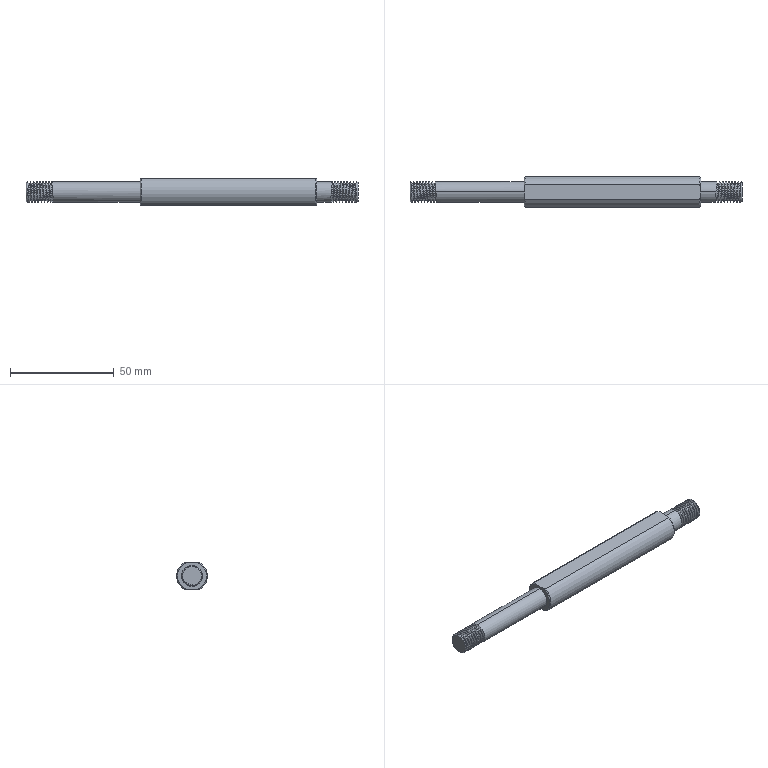Part | SolidWorks | features Chamfer 1, ICE 1, MirrorPattern 1, Revolution 1, SweepThread 1 | 1 solid | 62 faces | box 160 x 15 x 13 mm | volume 19723 mm3 | cylinder 38 | plane 10 | cone 8 | spline 6 | commonest cylinder face diameters 10 x36 15 x2